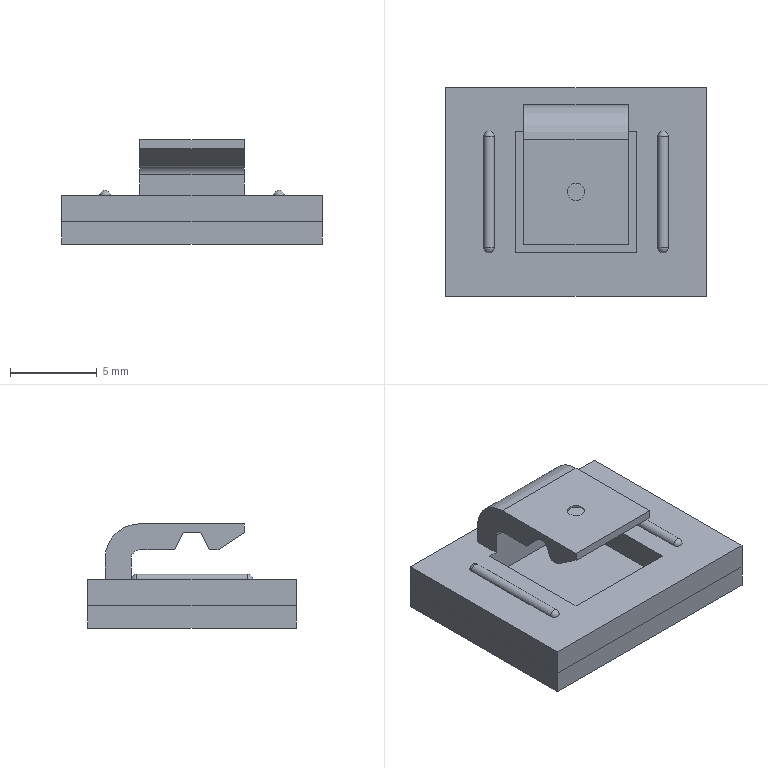Part | STEP file | Mount electronic clip black colour part | 2 solids | 38 faces | box 15 x 12 x 6 mm | volume 501.316 mm3 | plane 28 | cylinder 6 | sphere 4 | commonest cylinder face diameters 1 x3 0.6 x2 4 x1